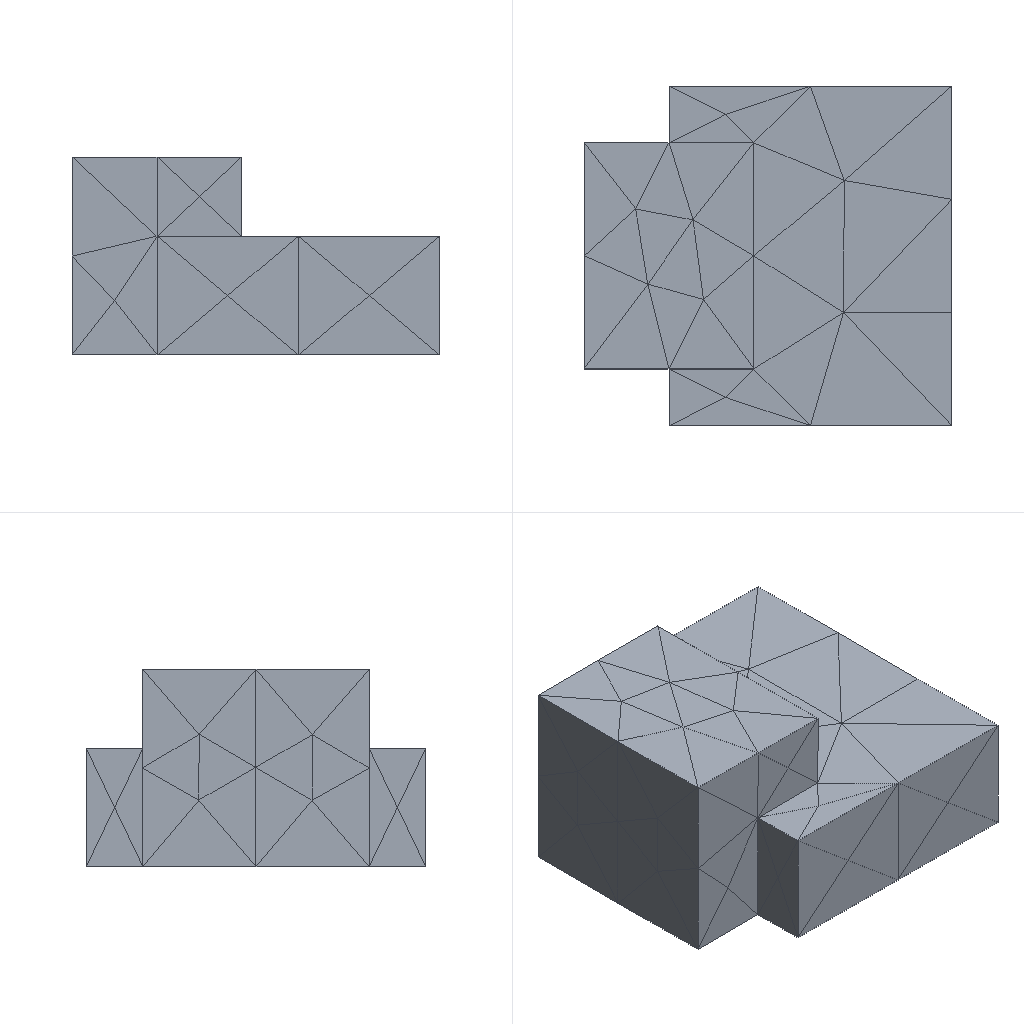Simulation study | ansys mapdl
Set-up summary:
category,name,step,type,value,unit,region
solver,ansys_mapdl
units,mm-N-s-tonne (MPa),,inferred,E=210000 density=
analysis,model,,static
mesh,nodes,,,409
mesh,elements,,,183
element_type,SOLID187,,,183
material,mat 1,,E,210000
material,mat 1,,nu,0.3
load,,model,body load temp,,,all
load,,model,force,"1000 [dir=(0, 0, -1) n=82]",,node list
bc,,model,fixed,"[dofs=UX,UY,UZ n=554]",,node list
Ansys APDL input file, long lists of numbers shortened:
/COM,ANSYS RELEASE 2026 R1           BUILD 26.1      UP20260202       09:08:46
/PREP7
/NOPR
/TITLE,2
ANTYPE, 0
*IF,_CDRDOFF,EQ,1,THEN     !if solid model was read in
_CDRDOFF=             !reset flag, numoffs already performed
*ELSE              !offset database for the following FE model
NUMOFF,NODE,      409
NUMOFF,ELEM,      183
NUMOFF,MAT ,        1
NUMOFF,TYPE,        1
*ENDIF
*SET,_RETURN ,  0.
*SET,_STATUS ,  0.
*SET,_UIQR   ,  82.
*SET,__FLOATPARAMETER__,  409.
DOF,DELETE
ETBLOCK,        1,        1
(2i9,19a9)
        1      187        0        0        0        0        0        0        0        0        0        0        0        0        0        0        0        0        0        0        0
       -1
NBLOCK,6,SOLID,       409,       409
(3i9,6e21.13e3)
        1        0        0 5.5000000000000E+001-1.2000000000000E+001
! (408 more lines like these left out)
N,UNBL,LOC,       -1,
EBLOCK,19,SOLID,       183,       183
(19i10)
         1         1         1         1         0         0         0         0        10         0         1       295        20        81        22       297       141       298       299
! (365 more lines like these left out)
        -1
MPTEMP,UNBL, 1, 1,  0.    ,
MPDATA,UNBL, 1,EX  ,       1, 1,  210000.000    ,
MPTEMP,UNBL, 1, 1,  0.    ,
MPDATA,UNBL, 1,NUXY,       1, 1, 0.3    ,
MPTEMP,UNBL, 1, 1,  0.    ,
MPDATA,UNBL, 1,PRXY,       1, 1, 0.3    ,
EXTOPT,ATTR,      0,      0,      0
EXTOPT,ESIZE,  0,  0.
EXTOPT,ACLEAR,      0
TREF,  0.
IRLF,  0
BFUNIF,TEMP,_TINY
ACEL,  0.    ,  0.    ,  0.
OMEGA,  0.    ,  0.    ,  0.
DOMEGA,  0.    ,  0.    ,  0.
CGLOC,  0.    ,  0.    ,  0.
CGOMEGA,  0.    ,  0.    ,  0.
DCGOMG,  0.    ,  0.    ,  0.
KUSE,     0
TIME,  0.
ALPHAD,  0.
BETAD,  0.
DMPRAT,  0.
DMPSTR,  0.
CRPLIM, 0.1    ,   0
CRPLIM,  0.    ,   1
NCNV,     0, 1.000000000E+12,     0,  0.    ,  0.
NEQIT,     0
ERESX,DEFA
DBLOCK,       554
(i9,a6,2(pg16.9))
        1  UX    0.00000000      0.00000000
! (553 more lines like these left out)
       -1
FBLOCK,        82
(i9,a6,2(pg16.9))
      188  FZ   -12.1951220      0.00000000
! (81 more lines like these left out)
       -1
/GO
FINISH
Results summary:
result,analysis_type_db,,,static,unstated
result,n_sets,,,1,unstated
result,load_steps[0].set,load_step=1,,1,unstated
result,load_steps[0].substep,load_step=1,,1,unstated
result,load_steps[0].time,load_step=1,,1,unstated
result,load_steps[0].freq,load_step=1,,1,unstated
result,load_steps[0].max_usum,load_step=1,,0.0004593,unstated
result,load_steps[0].max_seqv,load_step=1,,11.258,unstated
result,load_steps[0].reaction_sum.FX,load_step=1,,-2.39595e-11,unstated
result,load_steps[0].reaction_sum.FY,load_step=1,,-1.01394e-11,unstated
result,load_steps[0].reaction_sum.FZ,load_step=1,,1000,unstated
result,load_steps[0].reaction_sum.MX,load_step=1,,0,unstated
result,load_steps[0].reaction_sum.MY,load_step=1,,0,unstated
result,load_steps[0].reaction_sum.MZ,load_step=1,,0,unstated
result,convergence,,,results present for all listed sets,unstated